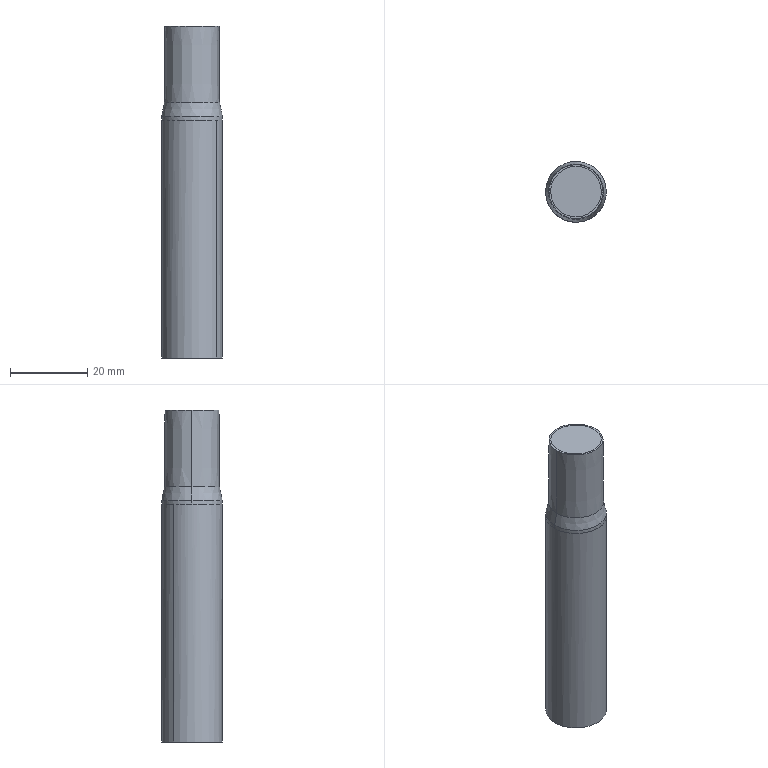Part | Creo | 1 solid | 11 faces | box 15.682 x 15.682 x 86.025 mm | volume 15818 mm3 | cone 4 | plane 3 | other 2 | cylinder 2 | commonest cylinder face diameters 15.678 x2